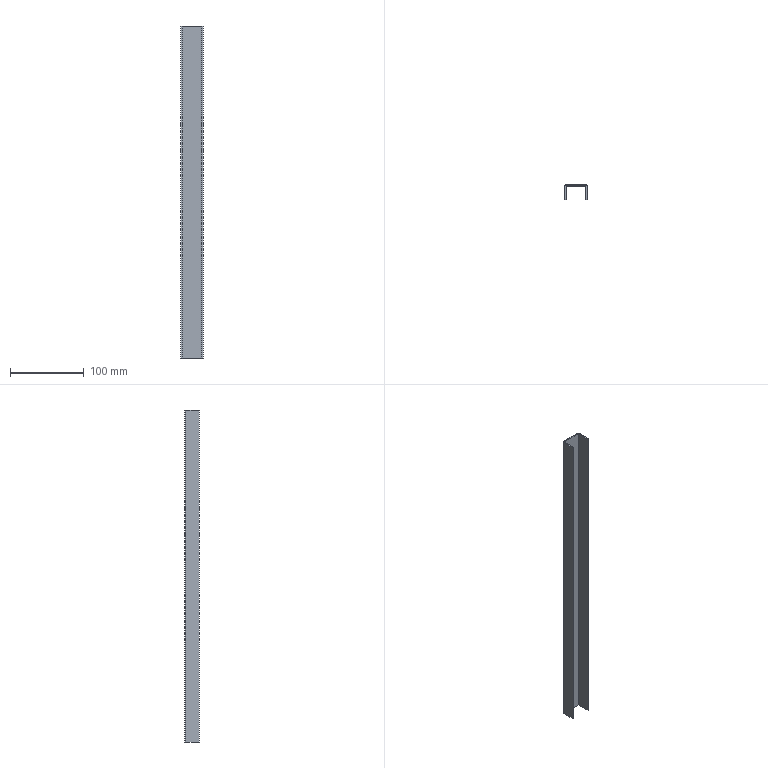Part | SolidWorks | features SplitBody 1 | 1 solid | 22 faces | box 30 x 20 x 450 mm | volume 44732 mm3 | plane 18 | cylinder 4 | commonest cylinder face diameters 0.2 x2 3.2 x2
STEP:
#1=CARTESIAN_POINT('',(-235.,28.4,185.));
#2=VERTEX_POINT('',#1);
#3=CARTESIAN_POINT('',(-236.5,28.4,185.));
#4=VERTEX_POINT('',#3);
#5=CARTESIAN_POINT('',(-235.,28.4,185.));
#6=DIRECTION('',(-1.,0.,0.));
#7=VECTOR('',#6,1000.);
#8=LINE('',#5,#7);
#9=EDGE_CURVE('',#2,#4,#8,.T.);
#10=ORIENTED_EDGE('',*,*,#9,.F.);
#11=CARTESIAN_POINT('',(-236.6,30.,185.));
#12=VERTEX_POINT('',#11);
#13=CARTESIAN_POINT('',(-236.6,28.4,185.));
#14=DIRECTION('',(0.,0.,1.));
#15=DIRECTION('',(0.,1.,0.));
#16=AXIS2_PLACEMENT_3D('',#13,#14,#15);
#17=CIRCLE('',#16,1.6);
#18=EDGE_CURVE('',#2,#12,#17,.T.);
#19=ORIENTED_EDGE('',*,*,#18,.T.);
#20=CARTESIAN_POINT('',(-236.6,28.5,185.));
#21=VERTEX_POINT('',#20);
#22=CARTESIAN_POINT('',(-236.6,28.5,185.));
#23=DIRECTION('',(0.,1.,0.));
#24=VECTOR('',#23,1000.);
#25=LINE('',#22,#24);
#26=EDGE_CURVE('',#21,#12,#25,.T.);
#27=ORIENTED_EDGE('',*,*,#26,.F.);
#28=CARTESIAN_POINT('',(-236.6,28.4,185.));
#29=DIRECTION('',(0.,0.,1.));
#30=DIRECTION('',(-1.,0.,0.));
#31=AXIS2_PLACEMENT_3D('',#28,#29,#30);
#32=CIRCLE('',#31,0.1);
#33=EDGE_CURVE('',#4,#21,#32,.T.);
#34=ORIENTED_EDGE('',*,*,#33,.F.);
#35=EDGE_LOOP('',(#10,#19,#27,#34));
#36=FACE_OUTER_BOUND('',#35,.T.);
#37=CARTESIAN_POINT('',(-235.,28.4,185.));
#38=DIRECTION('',(0.,0.,1.));
#39=DIRECTION('',(0.,-1.,0.));
#40=AXIS2_PLACEMENT_3D('',#37,#38,#39);
#41=PLANE('',#40);
#42=ADVANCED_FACE('',(#36),#41,.T.);
#43=CARTESIAN_POINT('',(-235.,10.,185.));
#44=VERTEX_POINT('',#43);
#45=CARTESIAN_POINT('',(-235.,10.,185.));
#46=DIRECTION('',(0.,1.,0.));
#47=VECTOR('',#46,1000.);
#48=LINE('',#45,#47);
#49=EDGE_CURVE('',#44,#2,#48,.T.);
#50=ORIENTED_EDGE('',*,*,#49,.T.);
#51=ORIENTED_EDGE('',*,*,#9,.T.);
#52=CARTESIAN_POINT('',(-236.5,10.,185.));
#53=VERTEX_POINT('',#52);
#54=CARTESIAN_POINT('',(-236.5,10.,185.));
#55=DIRECTION('',(0.,1.,0.));
#56=VECTOR('',#55,1000.);
#57=LINE('',#54,#56);
#58=EDGE_CURVE('',#53,#4,#57,.T.);
#59=ORIENTED_EDGE('',*,*,#58,.F.);
#60=CARTESIAN_POINT('',(-236.5,10.,185.));
#61=DIRECTION('',(1.,0.,0.));
#62=VECTOR('',#61,1000.);
#63=LINE('',#60,#62);
#64=EDGE_CURVE('',#53,#44,#63,.T.);
#65=ORIENTED_EDGE('',*,*,#64,.T.);
#66=EDGE_LOOP('',(#50,#51,#59,#65));
#67=FACE_OUTER_BOUND('',#66,.T.);
#68=CARTESIAN_POINT('',(-236.6,28.5,185.));
#69=DIRECTION('',(0.,0.,1.));
#70=DIRECTION('',(0.,-1.,0.));
#71=AXIS2_PLACEMENT_3D('',#68,#69,#70);
#72=PLANE('',#71);
#73=ADVANCED_FACE('',(#67),#72,.T.);
#74=CARTESIAN_POINT('',(-263.4,30.,185.));
#75=VERTEX_POINT('',#74);
#76=CARTESIAN_POINT('',(-263.4,28.5,185.));
#77=VERTEX_POINT('',#76);
#78=CARTESIAN_POINT('',(-263.4,30.,185.));
#79=DIRECTION('',(0.,-1.,0.));
#80=VECTOR('',#79,1000.);
#81=LINE('',#78,#80);
#82=EDGE_CURVE('',#75,#77,#81,.T.);
#83=ORIENTED_EDGE('',*,*,#82,.F.);
#84=CARTESIAN_POINT('',(-265.,28.4,185.));
#85=VERTEX_POINT('',#84);
#86=CARTESIAN_POINT('',(-263.4,28.4,185.));
#87=DIRECTION('',(0.,0.,1.));
#88=DIRECTION('',(0.,1.,0.));
#89=AXIS2_PLACEMENT_3D('',#86,#87,#88);
#90=CIRCLE('',#89,1.6);
#91=EDGE_CURVE('',#75,#85,#90,.T.);
#92=ORIENTED_EDGE('',*,*,#91,.T.);
#93=CARTESIAN_POINT('',(-263.5,28.4,185.));
#94=VERTEX_POINT('',#93);
#95=CARTESIAN_POINT('',(-263.5,28.4,185.));
#96=DIRECTION('',(-1.,0.,0.));
#97=VECTOR('',#96,1000.);
#98=LINE('',#95,#97);
#99=EDGE_CURVE('',#94,#85,#98,.T.);
#100=ORIENTED_EDGE('',*,*,#99,.F.);
#101=CARTESIAN_POINT('',(-263.4,28.4,185.));
#102=DIRECTION('',(0.,0.,1.));
#103=DIRECTION('',(-1.,0.,0.));
#104=AXIS2_PLACEMENT_3D('',#101,#102,#103);
#105=CIRCLE('',#104,0.1);
#106=EDGE_CURVE('',#77,#94,#105,.T.);
#107=ORIENTED_EDGE('',*,*,#106,.F.);
#108=EDGE_LOOP('',(#83,#92,#100,#107));
#109=FACE_OUTER_BOUND('',#108,.T.);
#110=CARTESIAN_POINT('',(-263.4,30.,185.));
#111=DIRECTION('',(0.,0.,1.));
#112=DIRECTION('',(0.,-1.,0.));
#113=AXIS2_PLACEMENT_3D('',#110,#111,#112);
#114=PLANE('',#113);
#115=ADVANCED_FACE('',(#109),#114,.T.);
#116=CARTESIAN_POINT('',(-235.,30.,185.));
#117=DIRECTION('',(-1.,0.,0.));
#118=VECTOR('',#117,1000.);
#119=LINE('',#116,#118);
#120=EDGE_CURVE('',#12,#75,#119,.T.);
#121=ORIENTED_EDGE('',*,*,#120,.T.);
#122=ORIENTED_EDGE('',*,*,#82,.T.);
#123=CARTESIAN_POINT('',(-235.,28.5,185.));
#124=DIRECTION('',(-1.,0.,0.));
#125=VECTOR('',#124,1000.);
#126=LINE('',#123,#125);
#127=EDGE_CURVE('',#21,#77,#126,.T.);
#128=ORIENTED_EDGE('',*,*,#127,.F.);
#129=ORIENTED_EDGE('',*,*,#26,.T.);
#130=EDGE_LOOP('',(#121,#122,#128,#129));
#131=FACE_OUTER_BOUND('',#130,.T.);
#132=CARTESIAN_POINT('',(-263.5,28.4,185.));
#133=DIRECTION('',(0.,0.,1.));
#134=DIRECTION('',(0.,-1.,0.));
#135=AXIS2_PLACEMENT_3D('',#132,#133,#134);
#136=PLANE('',#135);
#137=ADVANCED_FACE('',(#131),#136,.T.);
#138=CARTESIAN_POINT('',(-263.5,10.,-265.));
#139=VERTEX_POINT('',#138);
#140=CARTESIAN_POINT('',(-263.5,28.4,-265.));
#141=VERTEX_POINT('',#140);
#142=CARTESIAN_POINT('',(-263.5,30.,-265.));
#143=DIRECTION('',(0.,1.,0.));
#144=VECTOR('',#143,1000.);
#145=LINE('',#142,#144);
#146=EDGE_CURVE('',#139,#141,#145,.T.);
#147=ORIENTED_EDGE('',*,*,#146,.T.);
#148=CARTESIAN_POINT('',(-263.5,28.4,-301.056));
#149=DIRECTION('',(0.,0.,1.));
#150=VECTOR('',#149,1000.);
#151=LINE('',#148,#150);
#152=EDGE_CURVE('',#141,#94,#151,.T.);
#153=ORIENTED_EDGE('',*,*,#152,.T.);
#154=CARTESIAN_POINT('',(-263.5,10.,185.));
#155=VERTEX_POINT('',#154);
#156=CARTESIAN_POINT('',(-263.5,30.,185.));
#157=DIRECTION('',(0.,-1.,0.));
#158=VECTOR('',#157,1000.);
#159=LINE('',#156,#158);
#160=EDGE_CURVE('',#94,#155,#159,.T.);
#161=ORIENTED_EDGE('',*,*,#160,.T.);
#162=CARTESIAN_POINT('',(-263.5,10.,-301.056));
#163=DIRECTION('',(0.,0.,1.));
#164=VECTOR('',#163,1000.);
#165=LINE('',#162,#164);
#166=EDGE_CURVE('',#139,#155,#165,.T.);
#167=ORIENTED_EDGE('',*,*,#166,.F.);
#168=EDGE_LOOP('',(#147,#153,#161,#167));
#169=FACE_OUTER_BOUND('',#168,.T.);
#170=CARTESIAN_POINT('',(-263.5,30.,-301.056));
#171=DIRECTION('',(-1.,0.,0.));
#172=DIRECTION('',(0.,0.,1.));
#173=AXIS2_PLACEMENT_3D('',#170,#171,#172);
#174=PLANE('',#173);
#175=ADVANCED_FACE('',(#169),#174,.F.);
#176=CARTESIAN_POINT('',(-265.,10.,-265.));
#177=VERTEX_POINT('',#176);
#178=CARTESIAN_POINT('',(-265.,10.,185.));
#179=VERTEX_POINT('',#178);
#180=CARTESIAN_POINT('',(-265.,10.,-301.056));
#181=DIRECTION('',(0.,0.,1.));
#182=VECTOR('',#181,1000.);
#183=LINE('',#180,#182);
#184=EDGE_CURVE('',#177,#179,#183,.T.);
#185=ORIENTED_EDGE('',*,*,#184,.F.);
#186=CARTESIAN_POINT('',(-263.5,10.,-265.));
#187=DIRECTION('',(-1.,0.,0.));
#188=VECTOR('',#187,1000.);
#189=LINE('',#186,#188);
#190=EDGE_CURVE('',#139,#177,#189,.T.);
#191=ORIENTED_EDGE('',*,*,#190,.F.);
#192=ORIENTED_EDGE('',*,*,#166,.T.);
#193=CARTESIAN_POINT('',(-265.,10.,185.));
#194=DIRECTION('',(1.,0.,0.));
#195=VECTOR('',#194,1000.);
#196=LINE('',#193,#195);
#197=EDGE_CURVE('',#179,#155,#196,.T.);
#198=ORIENTED_EDGE('',*,*,#197,.F.);
#199=EDGE_LOOP('',(#185,#191,#192,#198));
#200=FACE_OUTER_BOUND('',#199,.T.);
#201=CARTESIAN_POINT('',(-265.,10.,-301.056));
#202=DIRECTION('',(0.,-1.,0.));
#203=DIRECTION('',(0.,0.,-1.));
#204=AXIS2_PLACEMENT_3D('',#201,#202,#203);
#205=PLANE('',#204);
#206=ADVANCED_FACE('',(#200),#205,.T.);
#207=CARTESIAN_POINT('',(-265.,28.4,-265.));
#208=VERTEX_POINT('',#207);
#209=CARTESIAN_POINT('',(-265.,28.4,-301.056));
#210=DIRECTION('',(0.,0.,1.));
#211=VECTOR('',#210,1000.);
#212=LINE('',#209,#211);
#213=EDGE_CURVE('',#208,#85,#212,.T.);
#214=ORIENTED_EDGE('',*,*,#213,.F.);
#215=CARTESIAN_POINT('',(-265.,30.,-265.));
#216=DIRECTION('',(0.,1.,0.));
#217=VECTOR('',#216,1000.);
#218=LINE('',#215,#217);
#219=EDGE_CURVE('',#177,#208,#218,.T.);
#220=ORIENTED_EDGE('',*,*,#219,.F.);
#221=ORIENTED_EDGE('',*,*,#184,.T.);
#222=CARTESIAN_POINT('',(-265.,30.,185.));
#223=DIRECTION('',(0.,-1.,0.));
#224=VECTOR('',#223,1000.);
#225=LINE('',#222,#224);
#226=EDGE_CURVE('',#85,#179,#225,.T.);
#227=ORIENTED_EDGE('',*,*,#226,.F.);
#228=EDGE_LOOP('',(#214,#220,#221,#227));
#229=FACE_OUTER_BOUND('',#228,.T.);
#230=CARTESIAN_POINT('',(-265.,30.,-301.056));
#231=DIRECTION('',(-1.,0.,0.));
#232=DIRECTION('',(0.,0.,1.));
#233=AXIS2_PLACEMENT_3D('',#230,#231,#232);
#234=PLANE('',#233);
#235=ADVANCED_FACE('',(#229),#234,.T.);
#236=CARTESIAN_POINT('',(-263.4,30.,-265.));
#237=VERTEX_POINT('',#236);
#238=CARTESIAN_POINT('',(-263.4,30.,-301.056));
#239=DIRECTION('',(0.,0.,1.));
#240=VECTOR('',#239,1000.);
#241=LINE('',#238,#240);
#242=EDGE_CURVE('',#237,#75,#241,.T.);
#243=ORIENTED_EDGE('',*,*,#242,.F.);
#244=CARTESIAN_POINT('',(-263.4,28.4,-265.));
#245=DIRECTION('',(0.,0.,-1.));
#246=DIRECTION('',(-1.,0.,0.));
#247=AXIS2_PLACEMENT_3D('',#244,#245,#246);
#248=CIRCLE('',#247,1.6);
#249=EDGE_CURVE('',#208,#237,#248,.T.);
#250=ORIENTED_EDGE('',*,*,#249,.F.);
#251=ORIENTED_EDGE('',*,*,#213,.T.);
#252=ORIENTED_EDGE('',*,*,#91,.F.);
#253=EDGE_LOOP('',(#243,#250,#251,#252));
#254=FACE_OUTER_BOUND('',#253,.T.);
#255=CARTESIAN_POINT('',(-263.4,28.4,-301.056));
#256=DIRECTION('',(0.,0.,1.));
#257=DIRECTION('',(0.,-1.,0.));
#258=AXIS2_PLACEMENT_3D('',#255,#256,#257);
#259=CYLINDRICAL_SURFACE('',#258,1.6);
#260=ADVANCED_FACE('',(#254),#259,.T.);
#261=CARTESIAN_POINT('',(-236.6,30.,-265.));
#262=VERTEX_POINT('',#261);
#263=CARTESIAN_POINT('',(-236.6,30.,-301.056));
#264=DIRECTION('',(0.,0.,1.));
#265=VECTOR('',#264,1000.);
#266=LINE('',#263,#265);
#267=EDGE_CURVE('',#262,#12,#266,.T.);
#268=ORIENTED_EDGE('',*,*,#267,.F.);
#269=CARTESIAN_POINT('',(-235.,30.,-265.));
#270=DIRECTION('',(1.,0.,0.));
#271=VECTOR('',#270,1000.);
#272=LINE('',#269,#271);
#273=EDGE_CURVE('',#237,#262,#272,.T.);
#274=ORIENTED_EDGE('',*,*,#273,.F.);
#275=ORIENTED_EDGE('',*,*,#242,.T.);
#276=ORIENTED_EDGE('',*,*,#120,.F.);
#277=EDGE_LOOP('',(#268,#274,#275,#276));
#278=FACE_OUTER_BOUND('',#277,.T.);
#279=CARTESIAN_POINT('',(-235.,30.,-301.056));
#280=DIRECTION('',(0.,1.,0.));
#281=DIRECTION('',(0.,0.,1.));
#282=AXIS2_PLACEMENT_3D('',#279,#280,#281);
#283=PLANE('',#282);
#284=ADVANCED_FACE('',(#278),#283,.T.);
#285=CARTESIAN_POINT('',(-235.,28.4,-265.));
#286=VERTEX_POINT('',#285);
#287=CARTESIAN_POINT('',(-235.,28.4,-301.056));
#288=DIRECTION('',(0.,0.,1.));
#289=VECTOR('',#288,1000.);
#290=LINE('',#287,#289);
#291=EDGE_CURVE('',#286,#2,#290,.T.);
#292=ORIENTED_EDGE('',*,*,#291,.F.);
#293=CARTESIAN_POINT('',(-236.6,28.4,-265.));
#294=DIRECTION('',(0.,0.,-1.));
#295=DIRECTION('',(-1.,0.,0.));
#296=AXIS2_PLACEMENT_3D('',#293,#294,#295);
#297=CIRCLE('',#296,1.6);
#298=EDGE_CURVE('',#262,#286,#297,.T.);
#299=ORIENTED_EDGE('',*,*,#298,.F.);
#300=ORIENTED_EDGE('',*,*,#267,.T.);
#301=ORIENTED_EDGE('',*,*,#18,.F.);
#302=EDGE_LOOP('',(#292,#299,#300,#301));
#303=FACE_OUTER_BOUND('',#302,.T.);
#304=CARTESIAN_POINT('',(-236.6,28.4,-301.056));
#305=DIRECTION('',(0.,0.,1.));
#306=DIRECTION('',(0.,-1.,0.));
#307=AXIS2_PLACEMENT_3D('',#304,#305,#306);
#308=CYLINDRICAL_SURFACE('',#307,1.6);
#309=ADVANCED_FACE('',(#303),#308,.T.);
#310=CARTESIAN_POINT('',(-235.,10.,-265.));
#311=VERTEX_POINT('',#310);
#312=CARTESIAN_POINT('',(-235.,10.,-301.056));
#313=DIRECTION('',(0.,0.,1.));
#314=VECTOR('',#313,1000.);
#315=LINE('',#312,#314);
#316=EDGE_CURVE('',#311,#44,#315,.T.);
#317=ORIENTED_EDGE('',*,*,#316,.F.);
#318=CARTESIAN_POINT('',(-235.,10.,-265.));
#319=DIRECTION('',(0.,-1.,0.));
#320=VECTOR('',#319,1000.);
#321=LINE('',#318,#320);
#322=EDGE_CURVE('',#286,#311,#321,.T.);
#323=ORIENTED_EDGE('',*,*,#322,.F.);
#324=ORIENTED_EDGE('',*,*,#291,.T.);
#325=ORIENTED_EDGE('',*,*,#49,.F.);
#326=EDGE_LOOP('',(#317,#323,#324,#325));
#327=FACE_OUTER_BOUND('',#326,.T.);
#328=CARTESIAN_POINT('',(-235.,10.,-301.056));
#329=DIRECTION('',(1.,0.,0.));
#330=DIRECTION('',(0.,0.,-1.));
#331=AXIS2_PLACEMENT_3D('',#328,#329,#330);
#332=PLANE('',#331);
#333=ADVANCED_FACE('',(#327),#332,.T.);
#334=CARTESIAN_POINT('',(-236.5,10.,-265.));
#335=VERTEX_POINT('',#334);
#336=CARTESIAN_POINT('',(-236.5,10.,-301.056));
#337=DIRECTION('',(0.,0.,1.));
#338=VECTOR('',#337,1000.);
#339=LINE('',#336,#338);
#340=EDGE_CURVE('',#335,#53,#339,.T.);
#341=ORIENTED_EDGE('',*,*,#340,.F.);
#342=CARTESIAN_POINT('',(-236.5,10.,-265.));
#343=DIRECTION('',(1.,0.,0.));
#344=VECTOR('',#343,1000.);
#345=LINE('',#342,#344);
#346=EDGE_CURVE('',#335,#311,#345,.T.);
#347=ORIENTED_EDGE('',*,*,#346,.T.);
#348=ORIENTED_EDGE('',*,*,#316,.T.);
#349=ORIENTED_EDGE('',*,*,#64,.F.);
#350=EDGE_LOOP('',(#341,#347,#348,#349));
#351=FACE_OUTER_BOUND('',#350,.T.);
#352=CARTESIAN_POINT('',(-236.5,10.,-301.056));
#353=DIRECTION('',(0.,-1.,0.));
#354=DIRECTION('',(0.,0.,-1.));
#355=AXIS2_PLACEMENT_3D('',#352,#353,#354);
#356=PLANE('',#355);
#357=ADVANCED_FACE('',(#351),#356,.T.);
#358=CARTESIAN_POINT('',(-236.5,28.4,-265.));
#359=VERTEX_POINT('',#358);
#360=CARTESIAN_POINT('',(-236.5,10.,-265.));
#361=DIRECTION('',(0.,-1.,0.));
#362=VECTOR('',#361,1000.);
#363=LINE('',#360,#362);
#364=EDGE_CURVE('',#359,#335,#363,.T.);
#365=ORIENTED_EDGE('',*,*,#364,.T.);
#366=ORIENTED_EDGE('',*,*,#340,.T.);
#367=ORIENTED_EDGE('',*,*,#58,.T.);
#368=CARTESIAN_POINT('',(-236.5,28.4,-301.056));
#369=DIRECTION('',(0.,0.,1.));
#370=VECTOR('',#369,1000.);
#371=LINE('',#368,#370);
#372=EDGE_CURVE('',#359,#4,#371,.T.);
#373=ORIENTED_EDGE('',*,*,#372,.F.);
#374=EDGE_LOOP('',(#365,#366,#367,#373));
#375=FACE_OUTER_BOUND('',#374,.T.);
#376=CARTESIAN_POINT('',(-236.5,10.,-301.056));
#377=DIRECTION('',(1.,0.,0.));
#378=DIRECTION('',(0.,0.,-1.));
#379=AXIS2_PLACEMENT_3D('',#376,#377,#378);
#380=PLANE('',#379);
#381=ADVANCED_FACE('',(#375),#380,.F.);
#382=CARTESIAN_POINT('',(-236.6,28.5,-265.));
#383=VERTEX_POINT('',#382);
#384=CARTESIAN_POINT('',(-236.6,28.4,-265.));
#385=DIRECTION('',(0.,0.,-1.));
#386=DIRECTION('',(1.,0.,0.));
#387=AXIS2_PLACEMENT_3D('',#384,#385,#386);
#388=CIRCLE('',#387,0.1);
#389=EDGE_CURVE('',#383,#359,#388,.T.);
#390=ORIENTED_EDGE('',*,*,#389,.T.);
#391=ORIENTED_EDGE('',*,*,#372,.T.);
#392=ORIENTED_EDGE('',*,*,#33,.T.);
#393=CARTESIAN_POINT('',(-236.6,28.5,-301.056));
#394=DIRECTION('',(0.,0.,1.));
#395=VECTOR('',#394,1000.);
#396=LINE('',#393,#395);
#397=EDGE_CURVE('',#383,#21,#396,.T.);
#398=ORIENTED_EDGE('',*,*,#397,.F.);
#399=EDGE_LOOP('',(#390,#391,#392,#398));
#400=FACE_OUTER_BOUND('',#399,.T.);
#401=CARTESIAN_POINT('',(-236.6,28.4,-301.056));
#402=DIRECTION('',(0.,0.,1.));
#403=DIRECTION('',(0.,-1.,0.));
#404=AXIS2_PLACEMENT_3D('',#401,#402,#403);
#405=CYLINDRICAL_SURFACE('',#404,0.1);
#406=ADVANCED_FACE('',(#400),#405,.F.);
#407=CARTESIAN_POINT('',(-263.4,28.5,-265.));
#408=VERTEX_POINT('',#407);
#409=CARTESIAN_POINT('',(-235.,28.5,-265.));
#410=DIRECTION('',(1.,0.,0.));
#411=VECTOR('',#410,1000.);
#412=LINE('',#409,#411);
#413=EDGE_CURVE('',#408,#383,#412,.T.);
#414=ORIENTED_EDGE('',*,*,#413,.T.);
#415=ORIENTED_EDGE('',*,*,#397,.T.);
#416=ORIENTED_EDGE('',*,*,#127,.T.);
#417=CARTESIAN_POINT('',(-263.4,28.5,-301.056));
#418=DIRECTION('',(0.,0.,1.));
#419=VECTOR('',#418,1000.);
#420=LINE('',#417,#419);
#421=EDGE_CURVE('',#408,#77,#420,.T.);
#422=ORIENTED_EDGE('',*,*,#421,.F.);
#423=EDGE_LOOP('',(#414,#415,#416,#422));
#424=FACE_OUTER_BOUND('',#423,.T.);
#425=CARTESIAN_POINT('',(-235.,28.5,-301.056));
#426=DIRECTION('',(0.,1.,0.));
#427=DIRECTION('',(0.,0.,1.));
#428=AXIS2_PLACEMENT_3D('',#425,#426,#427);
#429=PLANE('',#428);
#430=ADVANCED_FACE('',(#424),#429,.F.);
#431=CARTESIAN_POINT('',(-263.4,28.4,-265.));
#432=DIRECTION('',(0.,0.,-1.));
#433=DIRECTION('',(1.,0.,0.));
#434=AXIS2_PLACEMENT_3D('',#431,#432,#433);
#435=CIRCLE('',#434,0.1);
#436=EDGE_CURVE('',#141,#408,#435,.T.);
#437=ORIENTED_EDGE('',*,*,#436,.T.);
#438=ORIENTED_EDGE('',*,*,#421,.T.);
#439=ORIENTED_EDGE('',*,*,#106,.T.);
#440=ORIENTED_EDGE('',*,*,#152,.F.);
#441=EDGE_LOOP('',(#437,#438,#439,#440));
#442=FACE_OUTER_BOUND('',#441,.T.);
#443=CARTESIAN_POINT('',(-263.4,28.4,-301.056));
#444=DIRECTION('',(0.,0.,1.));
#445=DIRECTION('',(0.,-1.,0.));
#446=AXIS2_PLACEMENT_3D('',#443,#444,#445);
#447=CYLINDRICAL_SURFACE('',#446,0.1);
#448=ADVANCED_FACE('',(#442),#447,.F.);
#449=ORIENTED_EDGE('',*,*,#160,.F.);
#450=ORIENTED_EDGE('',*,*,#99,.T.);
#451=ORIENTED_EDGE('',*,*,#226,.T.);
#452=ORIENTED_EDGE('',*,*,#197,.T.);
#453=EDGE_LOOP('',(#449,#450,#451,#452));
#454=FACE_OUTER_BOUND('',#453,.T.);
#455=CARTESIAN_POINT('',(-263.4,28.4,185.));
#456=DIRECTION('',(0.,0.,-1.));
#457=DIRECTION('',(0.,-1.,0.));
#458=AXIS2_PLACEMENT_3D('',#455,#456,#457);
#459=PLANE('',#458);
#460=ADVANCED_FACE('',(#454),#459,.F.);
#461=CARTESIAN_POINT('',(-263.5,28.4,-265.));
#462=DIRECTION('',(-1.,0.,0.));
#463=VECTOR('',#462,1000.);
#464=LINE('',#461,#463);
#465=EDGE_CURVE('',#141,#208,#464,.T.);
#466=ORIENTED_EDGE('',*,*,#465,.F.);
#467=ORIENTED_EDGE('',*,*,#146,.F.);
#468=ORIENTED_EDGE('',*,*,#190,.T.);
#469=ORIENTED_EDGE('',*,*,#219,.T.);
#470=EDGE_LOOP('',(#466,#467,#468,#469));
#471=FACE_OUTER_BOUND('',#470,.T.);
#472=CARTESIAN_POINT('',(-263.5,30.,-265.));
#473=DIRECTION('',(0.,0.,1.));
#474=DIRECTION('',(0.,1.,0.));
#475=AXIS2_PLACEMENT_3D('',#472,#473,#474);
#476=PLANE('',#475);
#477=ADVANCED_FACE('',(#471),#476,.F.);
#478=CARTESIAN_POINT('',(-236.6,28.5,-265.));
#479=DIRECTION('',(0.,1.,0.));
#480=VECTOR('',#479,1000.);
#481=LINE('',#478,#480);
#482=EDGE_CURVE('',#383,#262,#481,.T.);
#483=ORIENTED_EDGE('',*,*,#482,.F.);
#484=ORIENTED_EDGE('',*,*,#413,.F.);
#485=CARTESIAN_POINT('',(-263.4,28.5,-265.));
#486=DIRECTION('',(0.,1.,0.));
#487=VECTOR('',#486,1000.);
#488=LINE('',#485,#487);
#489=EDGE_CURVE('',#408,#237,#488,.T.);
#490=ORIENTED_EDGE('',*,*,#489,.T.);
#491=ORIENTED_EDGE('',*,*,#273,.T.);
#492=EDGE_LOOP('',(#483,#484,#490,#491));
#493=FACE_OUTER_BOUND('',#492,.T.);
#494=CARTESIAN_POINT('',(-235.,28.5,-265.));
#495=DIRECTION('',(0.,0.,1.));
#496=DIRECTION('',(1.,0.,0.));
#497=AXIS2_PLACEMENT_3D('',#494,#495,#496);
#498=PLANE('',#497);
#499=ADVANCED_FACE('',(#493),#498,.F.);
#500=ORIENTED_EDGE('',*,*,#346,.F.);
#501=ORIENTED_EDGE('',*,*,#364,.F.);
#502=CARTESIAN_POINT('',(-236.5,28.4,-265.));
#503=DIRECTION('',(1.,0.,0.));
#504=VECTOR('',#503,1000.);
#505=LINE('',#502,#504);
#506=EDGE_CURVE('',#359,#286,#505,.T.);
#507=ORIENTED_EDGE('',*,*,#506,.T.);
#508=ORIENTED_EDGE('',*,*,#322,.T.);
#509=EDGE_LOOP('',(#500,#501,#507,#508));
#510=FACE_OUTER_BOUND('',#509,.T.);
#511=CARTESIAN_POINT('',(-236.5,10.,-265.));
#512=DIRECTION('',(0.,0.,1.));
#513=DIRECTION('',(0.,-1.,0.));
#514=AXIS2_PLACEMENT_3D('',#511,#512,#513);
#515=PLANE('',#514);
#516=ADVANCED_FACE('',(#510),#515,.F.);
#517=ORIENTED_EDGE('',*,*,#298,.T.);
#518=ORIENTED_EDGE('',*,*,#506,.F.);
#519=ORIENTED_EDGE('',*,*,#389,.F.);
#520=ORIENTED_EDGE('',*,*,#482,.T.);
#521=EDGE_LOOP('',(#517,#518,#519,#520));
#522=FACE_OUTER_BOUND('',#521,.T.);
#523=CARTESIAN_POINT('',(-236.6,28.4,-265.));
#524=DIRECTION('',(0.,0.,-1.));
#525=DIRECTION('',(-1.,0.,0.));
#526=AXIS2_PLACEMENT_3D('',#523,#524,#525);
#527=PLANE('',#526);
#528=ADVANCED_FACE('',(#522),#527,.T.);
#529=ORIENTED_EDGE('',*,*,#249,.T.);
#530=ORIENTED_EDGE('',*,*,#489,.F.);
#531=ORIENTED_EDGE('',*,*,#436,.F.);
#532=ORIENTED_EDGE('',*,*,#465,.T.);
#533=EDGE_LOOP('',(#529,#530,#531,#532));
#534=FACE_OUTER_BOUND('',#533,.T.);
#535=CARTESIAN_POINT('',(-263.4,28.4,-265.));
#536=DIRECTION('',(0.,0.,-1.));
#537=DIRECTION('',(-1.,0.,0.));
#538=AXIS2_PLACEMENT_3D('',#535,#536,#537);
#539=PLANE('',#538);
#540=ADVANCED_FACE('',(#534),#539,.T.);
#541=CLOSED_SHELL('',(#42,#73,#115,#137,#175,#206,#235,#260,#284,#309,#333,#357,#381,#406,#430,#448,#460,#477,#499,#516,#528,#540));
#542=MANIFOLD_SOLID_BREP('',#541);
#543=CARTESIAN_POINT('',(0.,0.,0.));
#544=DIRECTION('',(0.,0.,1.));
#545=DIRECTION('',(1.,0.,0.));
#546=AXIS2_PLACEMENT_3D('',#543,#544,#545);
#547=(LENGTH_UNIT()NAMED_UNIT(*)SI_UNIT(.MILLI.,.METRE.));
#548=UNCERTAINTY_MEASURE_WITH_UNIT(LENGTH_MEASURE(0.00001),#547,'','');
#549=(NAMED_UNIT(*)PLANE_ANGLE_UNIT()SI_UNIT($,.RADIAN.));
#550=(NAMED_UNIT(*)SI_UNIT($,.STERADIAN.)SOLID_ANGLE_UNIT());
#551=(GEOMETRIC_REPRESENTATION_CONTEXT(3)GLOBAL_UNCERTAINTY_ASSIGNED_CONTEXT((#548))GLOBAL_UNIT_ASSIGNED_CONTEXT((#547,#549,#550))REPRESENTATION_CONTEXT('',''));
#552=ADVANCED_BREP_SHAPE_REPRESENTATION('',(#542,#546),#551);